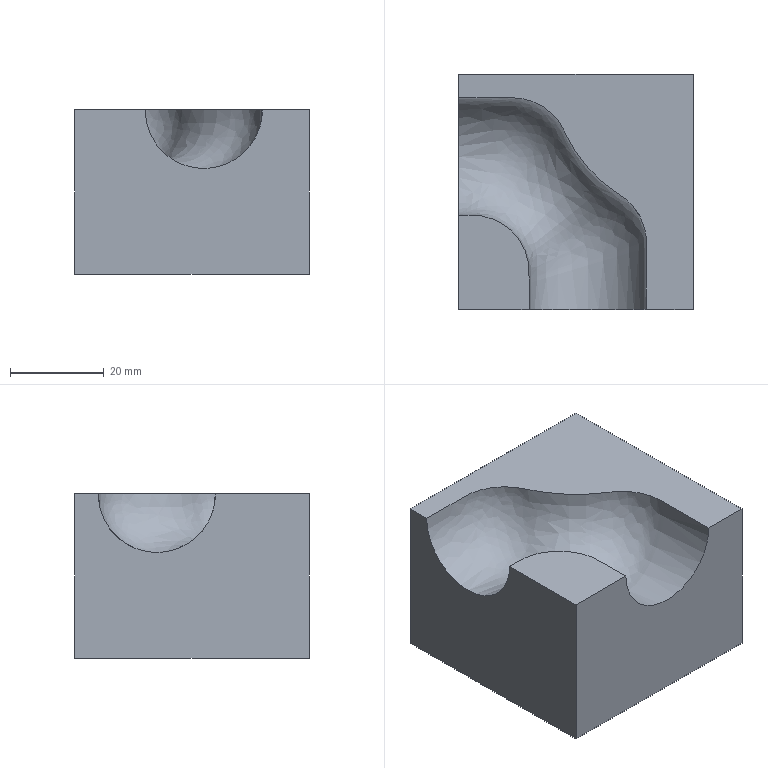NC program | NX | posted with a generic post | part box 50 x 50 x 35 mm
Lines 3839 to 4844 of 32931:
(CAVITY_MILL_COPY_COPY , TOOL : B8)
N7670 M6
N7672 G54
N7674 G17 G0 G90 X34.845 Y-4.368 S3000 M3
N7676 G43 Z10. H0
N7678 Z-7.838
N7680 G94 G1 Z-8.038 F2500.
N7682 X34.857 Y0.
N7684 G2 X35.006 Y13.847 R882.533
N7686 G3 X31.305 Y20.303 R7.249
N7688 G2 X28.081 Y22.278 R49.248
N7690 X19.859 Y31.804 R25.73
N7692 X18.247 Y35.369 R46.81
N7694 G3 X11.283 Y39.971 R7.347
N7696 G2 X0. Y39.853 R571.689
N7698 G1 X-4.372 Y39.851
N7700 Z-7.838
N7702 G0 Z-7.589
N7704 X-4.311 Y25.212
N7706 Z-7.838
N7708 G1 Z-8.038
N7710 X0. Y25.146
N7712 X3.416 Y25.094
N7714 X4.101 Y25.057
N7716 G2 X13.693 Y21.558 R20.121
N7718 G1 X14.194 Y21.229
N7720 G2 X19.247 Y13.693 R13.508
N7722 X19.933 Y8.897 R23.409
N7724 G1 X19.967 Y7.527
N7726 X20.119 Y2.483
N7728 G2 X20.144 Y0.02 R61.602
N7730 G1 X20.143 Y0.
N7732 X20.076 Y-4.422
N7734 Z-7.838
N7736 G0 Z-7.589
N7738 X34.763 Y-4.344
N7740 Z-7.986
N7742 G1 Z-8.186
N7744 X34.771 Y0.
N7746 G2 X34.941 Y13.811 R662.021
N7748 G3 X31.33 Y20.195 R7.162
N7750 G2 X29.007 Y21.566 R92.008
N7752 X20.863 Y29.828 R23.928
N7754 G1 X20.682 Y30.136
N7756 G2 X18.366 Y34.932 R31.522
N7758 G3 X14.378 Y39.273 R7.553
N7760 X11.346 Y39.897 R6.969
N7762 G2 X0. Y39.774 R553.614
N7764 G1 X-4.354 Y39.771
N7766 Z-7.986
N7768 G0 Z-7.738
N7770 X-4.296 Y25.295
N7772 Z-7.986
N7774 G1 Z-8.186
N7776 X0. Y25.229
N7778 X3.416 Y25.176
N7780 X4.101 Y25.139
N7782 G2 X13.353 Y21.914 R21.023
N7784 G1 X13.953 Y21.505
N7786 G2 X19.393 Y13.486 R13.189
N7788 X20.019 Y8.212 R25.068
N7790 G1 X20.038 Y7.527
N7792 X20.168 Y3.462
N7794 G2 X20.222 Y0.002 R106.996
N7796 G1 Y0.
N7798 X20.218 Y-4.359
N7800 Z-7.986
N7802 G0 Z-7.738
N7804 X34.677 Y-4.331
N7806 Z-8.135
N7808 G1 Z-8.335
N7810 X34.684 Y0.
N7812 G2 X34.861 Y13.693 R612.258
N7814 G3 X30.821 Y20.393 R7.191
N7816 G2 X23.468 Y26.025 R26.6
N7818 X18.565 Y34.247 R29.358
N7820 G1 X18.182 Y35.176
N7822 G3 X17.773 Y36.033 R8.85
N7824 X11.261 Y39.819 R7.256
N7826 G1 X8.897 Y39.774
N7828 X0.084 Y39.689
N7830 X0.
N7832 X-4.389 Y39.743
N7834 Z-8.135
N7836 G0 Z-7.886
N7838 X-4.401 Y25.253
N7840 Z-8.135
N7842 G1 Z-8.335
N7844 X0. Y25.309
N7846 X0.108
N7848 X3.416 Y25.258
N7850 X4.101 Y25.222
N7852 G2 X13.693 Y21.809 R21.352
N7854 G1 X13.946 Y21.642
N7856 G2 X19.308 Y14.16 R12.838
N7858 X20.073 Y8.897 R23.988
N7860 G1 X20.089 Y8.212
N7862 G2 X20.315 Y0. R255.107
N7864 G1 X20.364 Y-4.297
N7866 Z-8.135
N7868 G0 Z-7.886
N7870 X34.587 Y-4.317
N7872 Z-8.283
N7874 G1 Z-8.483
N7876 X34.598 Y0.
N7878 G2 X34.781 Y13.693 R630.965
N7880 G3 X30.821 Y20.288 R7.071
N7882 G2 X22.72 Y26.71 R25.753
N7884 X18.213 Y34.932 R30.316
N7886 G3 X14.378 Y39.097 R7.424
N7888 X10.953 Y39.738 R7.449
N7890 G2 X0. Y39.593 R410.331
N7892 G1 X-4.327
N7894 Z-8.283
N7896 G0 Z-8.035
N7898 X-4.378 Y25.353
N7900 Z-8.283
N7902 G1 Z-8.483
N7904 X0. Y25.409
N7906 G2 X4.786 Y25.235 R48.96
N7908 X13.733 Y21.914 R22.137
N7910 G1 X13.957 Y21.772
N7912 G2 X19.174 Y14.934 R12.414
N7914 X19.648 Y13.147 R14.01
N7916 X20.179 Y7.527 R28.502
N7918 X20.407 Y0. R162.24
N7920 G1 X20.438 Y-4.306
N7922 Z-8.283
N7924 G0 Z-8.035
N7926 X34.48 Y-4.31
N7928 Z-8.432
N7930 G1 Z-8.632
N7932 X34.498 Y0.
N7934 G2 X34.701 Y13.693 R642.154
N7936 G3 X30.821 Y20.183 R6.96
N7938 G2 X23.715 Y25.34 R26.88
N7940 X19.174 Y32.403 R25.633
N7942 X18.135 Y34.932 R25.774
N7944 G3 X10.953 Y39.651 R7.253
N7946 G2 X0. Y39.498 R331.815
N7948 G1 X-4.32 Y39.509
N7950 Z-8.432
N7952 G0 Z-8.183
N7954 X-4.394 Y25.413
N7956 Z-8.432
N7958 G1 Z-8.632
N7960 X0. Y25.515
N7962 G2 X5.472 Y25.231 R36.607
N7964 X14.378 Y21.652 R23.834
N7966 X19.643 Y13.693 R12.782
N7968 X20.217 Y8.897 R26.712
N7970 G1 X20.235 Y8.212
N7972 G2 X20.5 Y0. R183.782
N7974 G1 X20.543 Y-4.286
N7976 Z-8.432
N7978 G0 Z-8.183
N7980 X34.382 Y-4.279
N7982 Z-8.58
N7984 G1 Z-8.78
N7986 X34.397 Y0.
N7988 G2 X34.621 Y13.693 R527.549
N7990 G3 X30.821 Y20.078 R6.903
N7992 G2 X25.701 Y23.325 R29.624
N7994 X20.628 Y29.27 R20.008
N7996 X18.042 Y34.932 R38.227
N7998 G3 X10.953 Y39.562 R7.181
N8000 G2 X0. Y39.403 R291.829
N8002 G1 X-4.321 Y39.422
N8004 Z-8.58
N8006 G0 Z-8.332
N8008 X-4.319 Y25.577
N8010 Z-8.58
N8012 G1 Z-8.78
N8014 X0. Y25.619
N8016 X0.105 Y25.618
N8018 X3.416 Y25.552
N8020 X4.101 Y25.505
N8022 G2 X13.004 Y22.6 R22.932
N8024 G1 X13.428 Y22.372
N8026 G2 X19.619 Y14.257 R12.335
N8028 X20.302 Y8.897 R26.924
N8030 G1 X20.32 Y8.212
N8032 G2 X20.602 Y0.146 R203.997
N8034 G1 Y0.
N8036 X20.501 Y-4.393
N8038 Z-8.58
N8040 G0 Z-8.332
N8042 X34.281 Y-4.285
N8044 Z-8.729
N8046 G1 Z-8.929
N8048 X34.296 Y0.
N8050 G2 X34.533 Y13.693 R488.916
N8052 G3 X30.821 Y19.973 R6.874
N8054 G2 X26.312 Y22.674 R31.164
N8056 X20.486 Y29.267 R19.904
N8058 X17.949 Y34.932 R38.854
N8060 G3 X10.953 Y39.472 R7.118
N8062 G2 X0. Y39.295 R279.521
N8064 G1 X-4.296 Y39.309
N8066 Z-8.729
N8068 G0 Z-8.48
N8070 X-4.545 Y25.417
N8072 Z-8.729
N8074 G1 Z-8.929
N8076 X0. Y25.717
N8078 G2 X2.046 Y25.701 R13.953
N8080 X8.525 Y24.655 R20.15
N8082 X14.459 Y21.901 R25.653
N8084 X19.53 Y15.063 R11.764
N8086 X20.386 Y8.897 R26.389
N8088 G1 X20.405 Y8.212
N8090 G2 X20.72 Y0. R190.986
N8092 G1 X20.791 Y-4.215
N8094 Z-8.729
N8096 G0 Z-8.48
N8098 X34.157 Y-4.266
N8100 Z-8.877
N8102 G1 Z-9.077
N8104 X34.182 Y0.
N8106 G2 X34.436 Y13.624 R525.067
N8108 G3 X30.506 Y20.024 R6.829
N8110 G2 X23.689 Y24.655 R26.042
N8112 X19.555 Y30.771 R22.618
N8114 X17.9 Y34.787 R54.779
N8116 G3 X11.025 Y39.386 R7.019
N8118 G2 X0. Y39.183 R249.721
N8120 G1 X-4.283 Y39.198
N8122 Z-8.877
N8124 G0 Z-8.629
N8126 X-4.192 Y25.916
N8128 Z-8.877
N8130 G1 Z-9.077
N8132 X0. Y25.832
N8134 X3.416 Y25.763
N8136 X4.101 Y25.717
N8138 G2 X12.323 Y23.224 R24.487
N8140 G1 X13.297 Y22.744
N8142 G2 X18.181 Y18.489 R12.687
N8144 X20.035 Y13.405 R14.244
N8146 X20.517 Y7.527 R38.351
N8148 X20.835 Y0. R112.35
N8150 G1 X20.873 Y-4.226
N8152 Z-8.877
N8154 G0 Z-8.629
N8156 X34.027 Y-4.249
N8158 Z-9.026
N8160 G1 Z-9.226
N8162 X34.056 Y0.
N8164 G2 X34.343 Y13.693 R481.69
N8166 G3 X30.596 Y19.859 R6.737
N8168 G2 X25.546 Y22.843 R29.71
N8170 X20.387 Y28.829 R17.563
N8172 X17.804 Y34.819 R42.228
N8174 G3 X13.008 Y39.08 R7.095
N8176 G1 X12.323 Y39.211
N8178 X11.638 Y39.275
N8180 X10.953 Y39.279
N8182 X10.267 Y39.24
N8184 G2 X0. Y39.071 R341.518
N8186 G1 X-4.26 Y39.064
N8188 Z-9.026
N8190 G0 Z-8.777
N8192 X-4.18 Y26.022
N8194 Z-9.026
N8196 G1 Z-9.226
N8198 X0. Y25.938
N8200 X3.416 Y25.869
N8202 X4.101 Y25.823
N8204 G2 X12.473 Y23.285 R25.461
N8206 G1 X13.008 Y23.031
N8208 G2 X17.379 Y19.859 R13.32
N8210 X19.976 Y14.378 R12.158
N8212 X20.584 Y8.212 R35.727
N8214 X20.951 Y0. R122.67
N8216 G1 X20.997 Y-4.192
N8218 Z-9.026
N8220 G0 Z-8.777
N8222 X33.908 Y-4.206
N8224 Z-9.174
N8226 G1 Z-9.374
N8228 X33.93 Y0.
N8230 G2 X34.248 Y13.693 R381.492
N8232 G3 X30.35 Y19.859 R6.681
N8234 G2 X23.847 Y23.97 R26.462
N8236 X19.254 Y30.821 R20.698
N8238 X17.755 Y34.645 R77.801
N8240 G3 X11.016 Y39.177 R6.877
N8242 G2 X0. Y38.941 R302.278
N8244 G1 X-4.221 Y38.928
N8246 Z-9.174
N8248 G0 Z-8.926
N8250 X-4.192 Y26.116
N8252 Z-9.174
N8254 G1 Z-9.374
N8256 X0. Y26.049
N8258 X2.583 Y26.009
N8260 G2 X6.157 Y25.627 R19.868
N8262 X14.378 Y22.479 R32.502
N8264 X19.953 Y15.063 R10.891
N8266 X20.693 Y8.212 R36.879
N8268 X21.066 Y0. R118.131
N8270 G1 X21.111 Y-4.181
N8272 Z-9.174
N8274 G0 Z-8.926
N8276 X34.064 Y-4.432
N8278 Z-9.323
N8280 G1 Z-9.523
N8282 X33.804 Y0.
N8284 G2 X33.797 Y0.29 R3.979
N8286 X34.13 Y13.544 R619.416
N8288 G3 X30.136 Y19.84 R6.592
N8290 G2 X24.964 Y22.794 R28.266
N8292 X20.443 Y28.004 R15.023
N8294 X17.804 Y34.295 R39.827
N8296 G3 X10.953 Y39.07 R6.911
N8298 G2 X0. Y38.806 R246.092
N8300 G1 X-4.232 Y38.798
N8302 Z-9.323
N8304 G0 Z-9.074
N8306 X-4.168 Y26.255
N8308 Z-9.323
N8310 G1 Z-9.523
N8312 X0. Y26.188
N8314 X2.085 Y26.155
N8316 G2 X6.157 Y25.746 R24.322
N8318 X15.063 Y22.299 R35.904
N8320 X20.114 Y15.063 R10.767
N8322 X20.801 Y8.212 R44.395
N8324 X21.182 Y0. R114.174
N8326 G1 X21.224 Y-4.172
N8328 Z-9.323
N8330 G0 Z-9.074
N8332 X33.652 Y-4.182
N8334 Z-9.471
N8336 G1 Z-9.671
N8338 X33.679 Y0.
N8340 G2 X34.018 Y13.693 R374.58
N8342 G3 X30.136 Y19.691 R6.433
N8344 G2 X25.051 Y22.468 R31.983
N8346 X20.316 Y27.835 R14.067
N8348 X17.701 Y34.247 R44.142
N8350 G3 X10.953 Y38.951 R6.784
N8352 G2 X0.092 Y38.671 R223.521
N8354 G1 X0. Y38.672
N8356 X-4.301 Y38.781
N8358 Z-9.471
N8360 G0 Z-9.223
N8362 X-4.407 Y26.073
N8364 Z-9.471
N8366 G1 Z-9.671
N8368 X0. Y26.325
N8370 X0.143 Y26.331
N8372 G2 X6.157 Y25.865 R31.019
N8374 X15.063 Y22.519 R39.954
N8376 X20.115 Y15.748 R9.969
N8378 X20.91 Y8.212 R42.46
N8380 X21.317 Y0. R122.004
N8382 G1 X21.381 Y-4.125
N8384 Z-9.471
N8386 G0 Z-9.223
N8388 X33.52 Y-4.143
N8390 Z-9.62
N8392 G1 Z-9.82
N8394 X33.551 Y0.
N8396 G2 X33.903 Y13.693 R373.813
N8398 G3 X30.136 Y19.542 R6.277
N8400 G2 X24.975 Y22.248 R36.188
N8402 X19.983 Y28.024 R13.147
N8404 X17.575 Y34.247 R68.246
N8406 G3 X10.953 Y38.826 R6.632
N8408 G2 X0.063 Y38.536 R215.74
N8410 G1 X0.
N8412 X-4.25 Y38.611
N8414 Z-9.62
N8416 G0 Z-9.371
N8418 X-4.365 Y26.232
N8420 Z-9.62
N8422 G1 Z-9.82
N8424 X0. Y26.466
N8426 X0.193 Y26.472
N8428 G2 X4.786 Y26.246 R44.736
N8430 X12.323 Y23.939 R32.706
N8432 X17.337 Y21.229 R16.103
N8434 X20.297 Y15.748 R9.951
N8436 X21.019 Y8.212 R49.937
N8438 X21.462 Y0.155 R117.682
N8440 G1 Y0.
N8442 X21.353 Y-4.286
N8444 Z-9.62
N8446 G0 Z-9.371
N8448 X33.5 Y-4.231
N8450 Z-9.768
N8452 G1 Z-9.968
N8454 X33.394 Y0.
N8456 X33.393 Y0.119
N8458 G2 X33.795 Y13.425 R334.808
N8460 G3 X30.033 Y19.437 R6.196
N8462 G2 X25.014 Y21.914 R49.698
N8464 X19.859 Y27.797 R12.008
N8466 X17.45 Y34.247 R72.924
N8468 G3 X10.953 Y38.702 R6.525
N8470 G2 X0. Y38.401 R208.484
N8472 G1 X-4.142 Y38.395
N8474 X-4.161 Y26.582
N8476 X0. Y26.605
N8478 G2 X4.786 Y26.388 R47.203
N8480 X12.666 Y23.97 R37.355
N8482 X16.946 Y21.914 R18.618
N8484 X20.341 Y16.433 R8.888
N8486 X21.128 Y8.212 R49.896
N8488 X21.611 Y0.169 R96.283
N8490 G1 X21.61 Y0.
N8492 X21.473 Y-4.287
N8494 Z-9.768
N8496 G0 Z-9.52
N8498 X33.363 Y-4.246
N8500 Z-9.917
N8502 G1 Z-10.117
N8504 X33.235 Y0.
N8506 X33.234 Y0.132
N8508 G2 X33.677 Y13.3 R275.221
N8510 G3 X29.688 Y19.454 R6.2
N8512 G2 X23.829 Y22.34 R34.453
N8514 X20.054 Y26.749 R9.515
N8516 X17.381 Y34.062 R81.507
N8518 G3 X10.879 Y38.573 R6.441
N8520 G2 X0. Y38.242 R220.933
N8522 G1 X-4.088 Y38.219
N8524 X-4.266 Y26.584
N8526 X0. Y26.722
N8528 G2 X5.472 Y26.411 R30.75
N8530 X13.008 Y24.013 R46.549
N8532 X18.306 Y21.229 R13.909
N8534 X20.681 Y15.748 R9.956
N8536 X21.238 Y8.212 R73.863
N8538 X21.762 Y0. R78.24
N8540 G1 X21.808 Y-4.077
N8542 Z-9.917
N8544 G0 Z-9.668
N8546 X33.224 Y-4.245
N8548 Z-10.065
N8550 G1 Z-10.265
N8552 X33.076 Y0.
N8554 X33.074 Y0.14
N8556 G2 X33.542 Y13.008 R224.073
N8558 G3 X29.451 Y19.385 R6.135
N8560 G2 X23.71 Y21.987 R50.287
N8562 X20.028 Y26.054 R8.077
N8564 X17.432 Y33.562 R70.404
N8566 G3 X10.794 Y38.446 R6.467
N8568 G2 X0. Y38.073 R246.012
N8570 G1 X-4.037 Y38.023
N8572 X-4.303 Y26.667
N8574 X0. Y26.926
N8576 X0.166 Y26.933
N8578 G2 X6.157 Y26.423 R30.559
N8580 X13.008 Y24.213 R69.164
N8582 G1 X14.985 Y23.551
N8584 G2 X18.489 Y21.655 R11.592
N8586 X20.51 Y17.861 R7.466
N8588 G1 X20.795 Y16.433
N8590 X20.978 Y15.063
N8592 X21.337 Y8.897
N8594 G2 X21.911 Y0. R100.02
N8596 G1 X21.991 Y-4.027
N8598 Z-10.065
N8600 G0 Z-9.817
N8602 X32.885 Y-4.041
N8604 Z-10.214
N8606 G1 Z-10.414
N8608 X32.914 Y0.
N8610 G2 X33.411 Y13.213 R218.52
N8612 G3 X29.698 Y19.126 R5.937
N8614 G1 X23.97 Y21.423
N8616 X22.775 Y21.983
N8618 G2 X19.998 Y25.033 R5.375
N8620 X17.299 Y33.562 R116.831
N8622 G3 X10.704 Y38.309 R6.378
N8624 G2 X0.13 Y37.907 R184.144
N8626 G1 X0. Y37.909
N8628 X-4.175 Y38.038
N8630 X-4.18 Y26.954
N8632 X0. Y27.1
N8634 G2 X8.897 Y25.801 R25.118
N8636 X17.322 Y22.987 R5654.639
N8638 X20.364 Y19.785 R4.711
N8640 X21.165 Y14.904 R22.673
N8642 G1 X21.523 Y8.212
N8644 X21.751 Y5.979
N8646 G2 X22.092 Y0.213 R67.651
N8648 X22.089 Y0. R3.365
N8650 G1 X21.891 Y-4.228
N8652 Z-10.214
N8654 G0 Z-9.965
N8656 X32.927 Y-4.194
N8658 Z-10.362
N8660 G1 Z-10.562
N8662 X32.732 Y0.
N8664 X32.729 Y0.197
N8666 G2 X33.269 Y13.249 R236.003
N8668 G3 X29.829 Y18.856 R5.666
N8670 X21.405 Y21.579 R50.175
N8672 G1 X20.967 Y21.526
N8674 X21.098 Y18.489
N8676 G2 X21.666 Y8.212 R280.012
N8678 X22.276 Y0.222 R73.192
N8680 X22.274 Y0. R3.295
N8682 G1 X22.082 Y-4.191
N8684 Z-10.362
N8686 G0 Z-10.114
N8688 X32.474 Y-4.
N8690 Z-10.511
N8692 G1 Z-10.711
N8694 X32.53 Y0.
N8696 G2 X33.12 Y13.17 R213.441
N8698 G3 X29.708 Y18.729 R5.564
N8700 X23.088 Y20.617 R29.694
N8702 X21.581 Y19.36 R1.298
N8704 X21.808 Y8.212 R143.368
N8706 G2 X22.466 Y0. R60.798
N8708 G1 X22.515 Y-4.
N8710 Z-10.511
N8712 G0 Z-10.262
N8714 X32.67 Y-4.24
N8716 Z-10.659
N8718 G1 Z-10.859
N8720 X32.332 Y0.
N8722 G2 X32.322 Y0.319 R3.439
N8724 X32.968 Y13.053 R170.582
N8726 G3 X29.546 Y18.615 R5.471
N8728 X23.846 Y19.994 R20.674
N8730 X22.038 Y18.518 R1.66
N8732 X22.267 Y5.885 R50.797
N8734 G2 X22.664 Y0. R39.16
N8736 G1 X22.632 Y-4.
N8738 Z-10.659
N8740 G0 Z-10.411
N8742 X32.526 Y-4.254
N8744 Z-10.808
N8746 G1 Z-11.008
N8748 X32.122 Y0.
N8750 G2 X32.107 Y0.413 R3.484
N8752 X32.805 Y12.996 R200.434
N8754 G3 X29.167 Y18.583 R5.409
N8756 X24.434 Y19.512 R17.802
N8758 X22.408 Y17.9 R1.941
N8760 X22.338 Y6.842 R34.217
N8762 G2 X22.889 Y0.317 R48.785
N8764 X22.879 Y0. R3.28
N8766 G1 X22.544 Y-4.193
N8768 Z-10.808
N8770 G0 Z-10.559
N8772 X32.255 Y-4.174
N8774 Z-10.956
N8776 G1 Z-11.156
N8778 X31.895 Y0.
N8780 G2 X31.884 Y0.35 R3.249
N8782 X32.622 Y12.96 R172.715
N8784 G3 X29.107 Y18.397 R5.22
N8786 G1 X28.766 Y18.514
N8788 X26.025 Y19.042
N8790 X25.137 Y19.1
N8792 G3 X22.622 Y17.157 R2.405
N8794 X22.49 Y7.195 R28.099
N8796 G2 X23.118 Y0.31 R46.764
N8798 X23.108 Y0. R3.212
N8800 G1 X22.777 Y-4.151
N8802 Z-10.956
N8804 G0 Z-10.708
N8806 X31.571 Y-4.
N8808 Z-11.105
N8810 G1 Z-11.305
N8812 X31.634 Y0.
N8814 X31.645 Y0.676
N8816 G2 X32.453 Y12.83 R140.532
N8818 G3 X28.648 Y18.312 R5.081
N8820 G1 X28.081 Y18.455
N8822 G3 X24.655 Y18.595 R8.719
N8824 X22.757 Y16.33 R3.069
N8826 X22.701 Y7.129 R24.473
N8828 G2 X23.351 Y0. R38.864
N8830 G1 X23.345 Y-4.
N8832 Z-11.105
N8834 G0 Z-10.856
N8836 X32.002 Y-4.271
N8838 Z-11.253
N8840 G1 Z-11.453
N8842 X31.359 Y0.
N8844 G2 X31.321 Y0.654 R3.547
N8846 X32.26 Y12.651 R140.945
N8848 G3 X27.395 Y18.318 R5.059
N8850 X23.97 Y17.66 R4.334
N8852 X22.713 Y14.81 R5.939
N8854 X22.871 Y7.524 R21.311
N8856 G2 X23.645 Y0.408 R42.11
N8858 X23.628 Y0. R3.086
N8860 G1 X23.176 Y-4.123
N8862 Z-11.253
N8864 G0 Z-11.005
N8866 X30.997 Y-4.
N8868 Z-11.402
N8870 G1 Z-11.602
N8872 X31.054 Y0.
N8874 X31.064 Y0.676
N8876 G2 X32.047 Y12.62 R119.457
N8878 G3 X27.395 Y18.055 R4.803
N8880 X23.285 Y15.737 R3.543
N8882 G1 X23.061 Y15.063
N8884 G3 X23.102 Y7.527 R18.125
N8886 G2 X23.937 Y0.169 R35.764
N8888 G1 X23.932 Y0.
N8890 X23.688 Y-4.
N8892 Z-11.402
N8894 G0 Z-11.153
N8896 X31.141
N8898 Z-11.55
N8900 G1 Z-11.75
N8902 X30.699 Y0.
N8904 G2 X30.687 Y0.397 R2.533
N8906 X31.788 Y12.323 R132.333
N8908 G3 X24.655 Y17.12 R4.705
N8910 X23.172 Y14.378 R4.953
N8912 X23.351 Y7.527 R17.251
N8914 G2 X24.288 Y0. R33.955
N8916 G1 X24.336 Y-4.
N8918 Z-11.55
N8920 G0 Z-11.302
N8922 X30.907
N8924 Z-11.699
N8926 G1 Z-11.899
N8928 X30.313 Y0.
N8930 G2 X30.291 Y0.535 R2.555
N8932 X31.594 Y12.488 R131.103
N8934 G3 X24.655 Y16.607 R4.347
N8936 X23.295 Y13.732 R5.326
N8938 X23.695 Y7.205 R16.486
N8940 G2 X24.647 Y0. R28.188
N8942 G1 X24.656 Y-4.
N8944 Z-11.699
N8946 G0 Z-11.45
N8948 X30.696
N8950 Z-11.847
N8952 G1 Z-12.047
N8954 X29.89 Y0.
N8956 G2 X29.848 Y0.71 R2.549
N8958 G1 X30.069 Y3.416
N8960 X31.354 Y12.574
N8962 G3 X25.34 Y16.653 R4.048
N8964 X23.598 Y13.763 R4.655
N8966 X23.97 Y7.315 R14.212
N8968 G2 X25.103 Y0.559 R29.013
N8970 X25.067 Y0. R2.503
N8972 G1 X24.353 Y-4.
N8974 Z-11.847
N8976 G0 Z-11.599
N8978 X29.018
N8980 Z-11.996
N8982 G1 Z-12.196
N8984 X29.314 Y0.
N8986 G2 X31.043 Y12.034 R88.138
N8988 G3 X30.176 Y15.588 R4.197
N8990 X23.979 Y14.108 R3.548
N8992 X24.374 Y7.148 R12.708
N8994 G2 X25.653 Y0. R23.158
N8996 G1 X25.732 Y-4.
N8998 Z-11.996
N9000 G0 Z-11.747
N9002 X28.003
N9004 Z-12.144
N9006 G1 Z-12.344
N9008 X28.378 Y0.
N9010 X28.442 Y0.676
N9012 X30.791 Y12.323
N9014 G3 X24.805 Y15.063 R3.361
N9016 X24.655 Y7.564 R8.963
N9018 G2 X26.496 Y0. R22.148
N9020 G1 X26.745 Y-4.
N9022 Z-12.144
N9024 G0 Z-11.896
N9026 X29.1 Y9.117
N9028 Z-12.144
N9030 G3 X24.489 Y10.399 Z-12.493 R-3.
N9032 G1 X26.548 Y5.184
N9034 X27.395 Y3.868
N9036 X27.697 Y4.101
N9038 G3 X30.477 Y12.821 R20.818
N9040 X24.664 Y13.946 R2.977
N9042 X25.701 Y6.5 R8.947
N9044 G1 X26.548 Y5.184
N9046 X28.23 Y6.267
N9048 X27.263 Y7.776
N9050 Z-12.293
N9052 G0 Z-12.044
N9054 X29.274 Y14.909
N9056 Z-12.293
N9058 G1 X28.496 Y15.399 Z-12.317
N9060 X27.724 Y15.578 Z-12.337
N9062 X26.765 Y15.473 Z-12.363
N9064 X25.908 Y15.029 Z-12.388
N9066 X25.269 Y14.306 Z-12.413
N9068 X24.879 Y13.354 Z-12.44
N9070 X24.602 Y11.783 Z-12.482
N9072 X24.705 Y10.191 Z-12.524
N9074 X25.181 Y8.669 Z-12.566
N9076 X26.004 Y7.302 Z-12.607
N9078 X26.438 Y6.842 Z-12.624
N9080 X27.053 Y6.606 Z-12.641
N9082 X27.669 Y6.371
N9084 G3 X30.121 Y12.785 R11.622
N9086 X25.119 Y13.94 R2.601
N9088 X26.438 Y6.842 R6.665
N9090 G1 X27.053 Y6.606
N9092 X28.484 Y10.342
N9094 X27.684 Y10.599
N9096 Z-12.441
N9098 G0 Z-12.193
N9100 X29.627 Y12.27
N9102 Z-12.441
N9104 G1 X29.684 Y13.173 Z-12.465
N9106 X29.508 Y13.823 Z-12.482
N9108 X29.137 Y14.387 Z-12.5
N9110 X28.609 Y14.806 Z-12.518
N9112 X27.938 Y15.047 Z-12.536
N9114 X27.263 Y15.058 Z-12.554
N9116 X26.619 Y14.859 Z-12.572
N9118 X26.07 Y14.468 Z-12.589
N9120 X25.557 Y13.76 Z-12.612
N9122 X25.113 Y12.631 Z-12.644
N9124 X24.987 Y11.424 Z-12.676
N9126 X25.189 Y10.228 Z-12.708
N9128 X25.705 Y9.129 Z-12.739
N9130 X26.495 Y8.209 Z-12.771
N9132 X26.92 Y7.912 Z-12.785
N9134 X27.102 Y7.874 Z-12.79
N9136 X28.081 Y8.349
N9138 G3 X29.662 Y12.817 R8.641
N9140 X25.861 Y14.18 R2.102
N9142 X26.92 Y7.912 R4.458
N9144 G1 X27.102 Y7.874
N9146 X27.915 Y11.791
N9148 X27.513 Y11.882
N9150 Z-12.59
N9152 G0 Z-12.341
N9154 X26.816 Y9.507
N9156 Z-12.59
N9158 G1 Z-12.938
N9160 G3 X28.928 Y13.442 R2.84
N9162 X26.098 Y13.479 R1.553
N9164 G1 X25.735 Y12.703
N9166 G3 X26.71 Y9.49 R2.509
N9168 G1 X26.816 Y9.507
N9170 X26.126 Y13.447
N9172 Z-12.738
N9174 G0 Z-12.49
N9176 X27.117 Y10.871
N9178 Z-12.738
N9180 G1 Z-13.087
N9182 G3 X28.319 Y12.323 R1.059
N9184 X26.71 Y12.752 R0.846
N9186 X27.117 Y10.871 R1.059
N9188 G1 X27.549 Y12.824
N9190 Z-12.887
N9192 G0 Z10.
N9194 X-4.31 Y26.934
N9196 Z-10.362
N9198 G1 Z-10.562
N9200 X0. Y27.274
N9202 G2 X0.287 Y27.286 R3.647
N9204 X4.786 Y27.021 R38.279
N9206 X11.638 Y25.052 R52.115
N9208 G3 X19.174 Y23.321 R33.407
N9210 G1 X19.478 Y23.477
N9212 X19.179 Y26.025
N9214 X19.015 Y26.71
N9216 X17.165 Y33.562
N9218 X17.042 Y33.927
N9220 G3 X10.637 Y38.149 R6.217
N9222 G2 X0.054 Y37.746 R119.947
N9224 G1 X0. Y37.747
N9226 X-4.131 Y37.843
N9228 Z-10.362
N9230 G0 Z-10.114
N9232 X-4.212 Y27.208
N9234 Z-10.511
N9236 G1 Z-10.711
N9238 X0. Y27.42
N9240 G2 X9.164 Y26.025 R23.149
N9242 G3 X17.159 Y24.078 R39.264
N9244 X18.695 Y25.573 R1.362
N9246 G1 X18.498 Y27.395
N9248 X17.119 Y33.217
N9250 X16.939 Y33.778
N9252 G3 X10.626 Y37.992 R6.096
N9254 G2 X0.184 Y37.54 R130.118
N9256 G1 X0. Y37.544
N9258 X-4.188 Y37.766
N9260 Z-10.511
N9262 G0 Z-10.262
N9264 X-4.05 Y27.556
N9266 Z-10.659
N9268 G1 Z-10.859
N9270 X0. Y27.675
N9272 G2 X8.897 Y26.296 R24.696
N9274 G3 X15.763 Y24.629 R29.894
N9276 X17.868 Y25.34 R2.578
N9278 X18.107 Y27.474 R4.203
N9280 G1 X17.814 Y29.451
N9282 X17.058 Y32.876
N9284 X16.792 Y33.713
N9286 G3 X10.557 Y37.833 R5.948
N9288 G2 X0. Y37.328 R111.192
N9290 G1 X-4. Y37.327
N9292 Z-10.659
N9294 G0 Z-10.411
N9296 X-4.032 Y27.75
N9298 Z-10.808
N9300 G1 Z-11.008
N9302 X0. Y27.891
N9304 G2 X6.842 Y27.104 R23.153
N9306 G1 X12.02 Y25.529
N9308 G3 X15.909 Y25.112 R10.446
N9310 X17.731 Y27.166 R1.985
N9312 X16.672 Y33.562 R25.773
N9314 X10.267 Y37.644 R5.876
N9316 G2 X0. Y37.117 R93.901
N9318 G1 X-4. Y37.131
N9320 Z-10.808
N9322 G0 Z-10.559
N9324 X-4.027 Y27.936
N9326 Z-10.956
N9328 G1 Z-11.156
N9330 X0. Y28.095
N9332 G2 X8.897 Y26.658 R22.707
N9334 G3 X14.767 Y25.374 R21.382
N9336 X17.355 Y27.787 R2.409
N9338 X16.567 Y33.346 R20.631
N9340 X10.416 Y37.468 R5.726
N9342 G2 X0. Y36.903 R89.474
N9344 G1 X-4. Y36.92
N9346 Z-10.956
N9348 G0 Z-10.708
N9350 X-4.025 Y28.101
N9352 Z-11.105
N9354 G1 Z-11.305
N9356 X0. Y28.337
N9358 X0.027 Y28.339
N9360 G2 X8.212 Y27.082 R20.71
N9362 G3 X13.308 Y25.729 R34.567
N9364 X16.475 Y26.638 R3.692
N9366 X17.008 Y29.451 R4.589
N9368 X16.11 Y33.986 R11.679
N9370 X10.45 Y37.281 R5.418
N9372 G2 X0.331 Y36.626 R88.737
N9374 X0. Y36.64 R3.192
N9376 G1 X-4.151 Y37.042
N9378 Z-11.105
N9380 G0 Z-10.856
N9382 X-4.09 Y28.239
N9384 Z-11.253
N9386 G1 Z-11.453
N9388 X0. Y28.624
N9390 G2 X0.345 Y28.637 R3.063
N9392 G1 X1.677 Y28.612
N9394 G2 X7.88 Y27.414 R18.484
N9396 G3 X13.615 Y26.006 R24.355
N9398 X16.658 Y28.404 R2.736
N9400 X16.095 Y33.562 R11.612
N9402 X10.267 Y37.065 R5.394
N9404 G2 X0.676 Y36.357 R76.696
N9406 G1 X0. Y36.362
N9408 X-4. Y36.392
N9410 Z-11.253
N9412 G0 Z-11.005
N9414 Y28.713
N9416 Z-11.402
N9418 G1 Z-11.602
N9420 X0. Y28.913
N9422 G2 X7.708 Y27.71 R19.176
N9424 G3 X13.197 Y26.306 R25.956
N9426 X16.333 Y28.581 R2.786
N9428 X15.881 Y33.562 R9.545
N9430 X10.267 Y36.85 R5.233
N9432 G2 X0.173 Y36.039 R75.234
N9434 G1 X0. Y36.043
N9436 X-4. Y36.281
N9438 Z-11.402
N9440 G0 Z-11.153
N9442 Y29.084
N9444 Z-11.55
N9446 G1 Z-11.75
N9448 X0. Y29.261
N9450 G2 X7.775 Y27.955 R18.874
N9452 G3 X13.008 Y26.624 R21.224
N9454 X16.011 Y28.766 R2.768
N9456 X15.441 Y33.938 R7.625
N9458 X10.22 Y36.612 R4.914
N9460 G2 X0. Y35.72 R64.88
N9462 G1 X-4. Y35.688
N9464 Z-11.55
N9466 G0 Z-11.302
N9468 Y29.074
N9470 Z-11.699
N9472 G1 Z-11.899
N9474 X0. Y29.629
N9476 G2 X0.316 Y29.654 R2.571
N9478 X7.93 Y28.171 R18.878
N9480 G3 X12.836 Y26.962 R16.078
N9482 X15.672 Y28.852 R2.739
N9484 X14.467 Y34.932 R6.378
N9486 X10.267 Y36.389 R4.89
N9488 G1 X6.644 Y35.843
N9490 G2 X0. Y35.328 R46.178
N9492 G1 X-4. Y35.307
N9494 Z-11.699
N9496 G0 Z-11.45
N9498 Y29.676
N9500 Z-11.847
N9502 G1 Z-12.047
N9504 X0. Y30.099
N9506 G2 X0.202 Y30.11 R1.937
N9508 X8.212 Y28.354 R19.076
N9510 G3 X13.693 Y27.388 R10.974
N9512 X15.687 Y30.821 R3.297
N9514 X10.953 Y36.171 R4.929
N9516 G1 X10.267 Y36.124
N9518 X5.472 Y35.295
N9520 X4.786 Y35.216
N9522 X0. Y34.899
N9524 X-4. Y34.633
N9526 Z-11.847
N9528 G0 Z-11.599
N9530 Y30.577
N9532 Z-11.996
N9534 G1 Z-12.196
N9536 X0. Y30.645
N9538 G2 X7.527 Y28.973 R16.534
N9540 G3 X12.323 Y27.651 R13.563
N9542 X15.381 Y30.821 R2.835
N9544 X9.853 Y35.739 R4.528
N9546 G2 X0. Y34.387 R53.663
N9548 G1 X-4. Y34.212
N9550 Z-11.996
N9552 G0 Z-11.747
N9554 Y31.338
N9556 Z-12.144
N9558 G1 Z-12.344
N9560 X0. Y31.418
N9562 G2 X6.842 Y29.725 R13.573
N9564 G3 X12.096 Y27.997 R13.2
N9566 X14.988 Y30.22 R2.642
N9568 G1 X15.063 Y30.706
N9570 G3 X9.582 Y35.379 R4.278
N9572 G2 X0. Y33.392 R58.911
N9574 G1 X-4. Y32.904
N9576 Z-12.144
N9578 G0 Z-11.896
N9580 X8.101 Y29.78
N9582 Z-12.144
N9584 G3 X9.012 Y34.818 Z-12.493 R-3.08
N9586 G1 X3.984 Y32.628
N9588 X3.876 Y32.38
N9590 G3 X11.471 Y28.426 R16.268
N9592 X14.671 Y30.953 R2.641
N9594 G1 X14.679 Y31.338
N9596 G3 X10.022 Y35.111 R3.795
N9598 X4.092 Y32.876 R24.236
N9600 G1 X3.984 Y32.628
N9602 X7.65 Y31.027
N9604 X8.075 Y31.805
N9606 Z-12.293
N9608 G0 Z-12.044
N9610 X8.366 Y30.287
N9612 Z-12.293
N9614 G3 X9.367 Y34.422 Z-12.641 R-2.88
N9616 G1 X6.211 Y32.69
N9618 G3 X8.212 Y29.991 R3.314
N9620 X13.49 Y29.451 R5.082
N9622 X10.505 Y34.773 R3.281
N9624 X6.211 Y32.69 R7.654
N9626 G1 X8.992 Y29.814
N9628 X9.817 Y31.327
N9630 Z-12.441
N9632 G0 Z-12.193
N9634 X10.098 Y29.599
N9636 Z-12.441
N9638 G1 X10.42 Y29.487 Z-12.45
N9640 X11.672 Y29.475 Z-12.483
N9642 X12.862 Y29.863 Z-12.516
N9644 X13.258 Y30.136 Z-12.528
N9646 X13.463 Y30.498 Z-12.539
N9648 X13.66 Y31.545 Z-12.567
N9650 X13.467 Y32.593 Z-12.595
N9652 X12.908 Y33.5 Z-12.623
N9654 X12.266 Y34.03 Z-12.645
N9656 X11.27 Y34.407 Z-12.672
N9658 X10.205 Y34.399 Z-12.7
N9660 X9.214 Y34.007 Z-12.728
N9662 X8.897 Y33.738 Z-12.739
N9664 X8.586 Y33.648 Z-12.748
N9666 X8.076 Y33.263 Z-12.764
N9668 X7.736 Y32.721 Z-12.781
N9670 X7.674 Y32.403 Z-12.79
N9672 G3 X7.968 Y31.057 R1.736
N9674 X13.258 Y30.136 R3.836